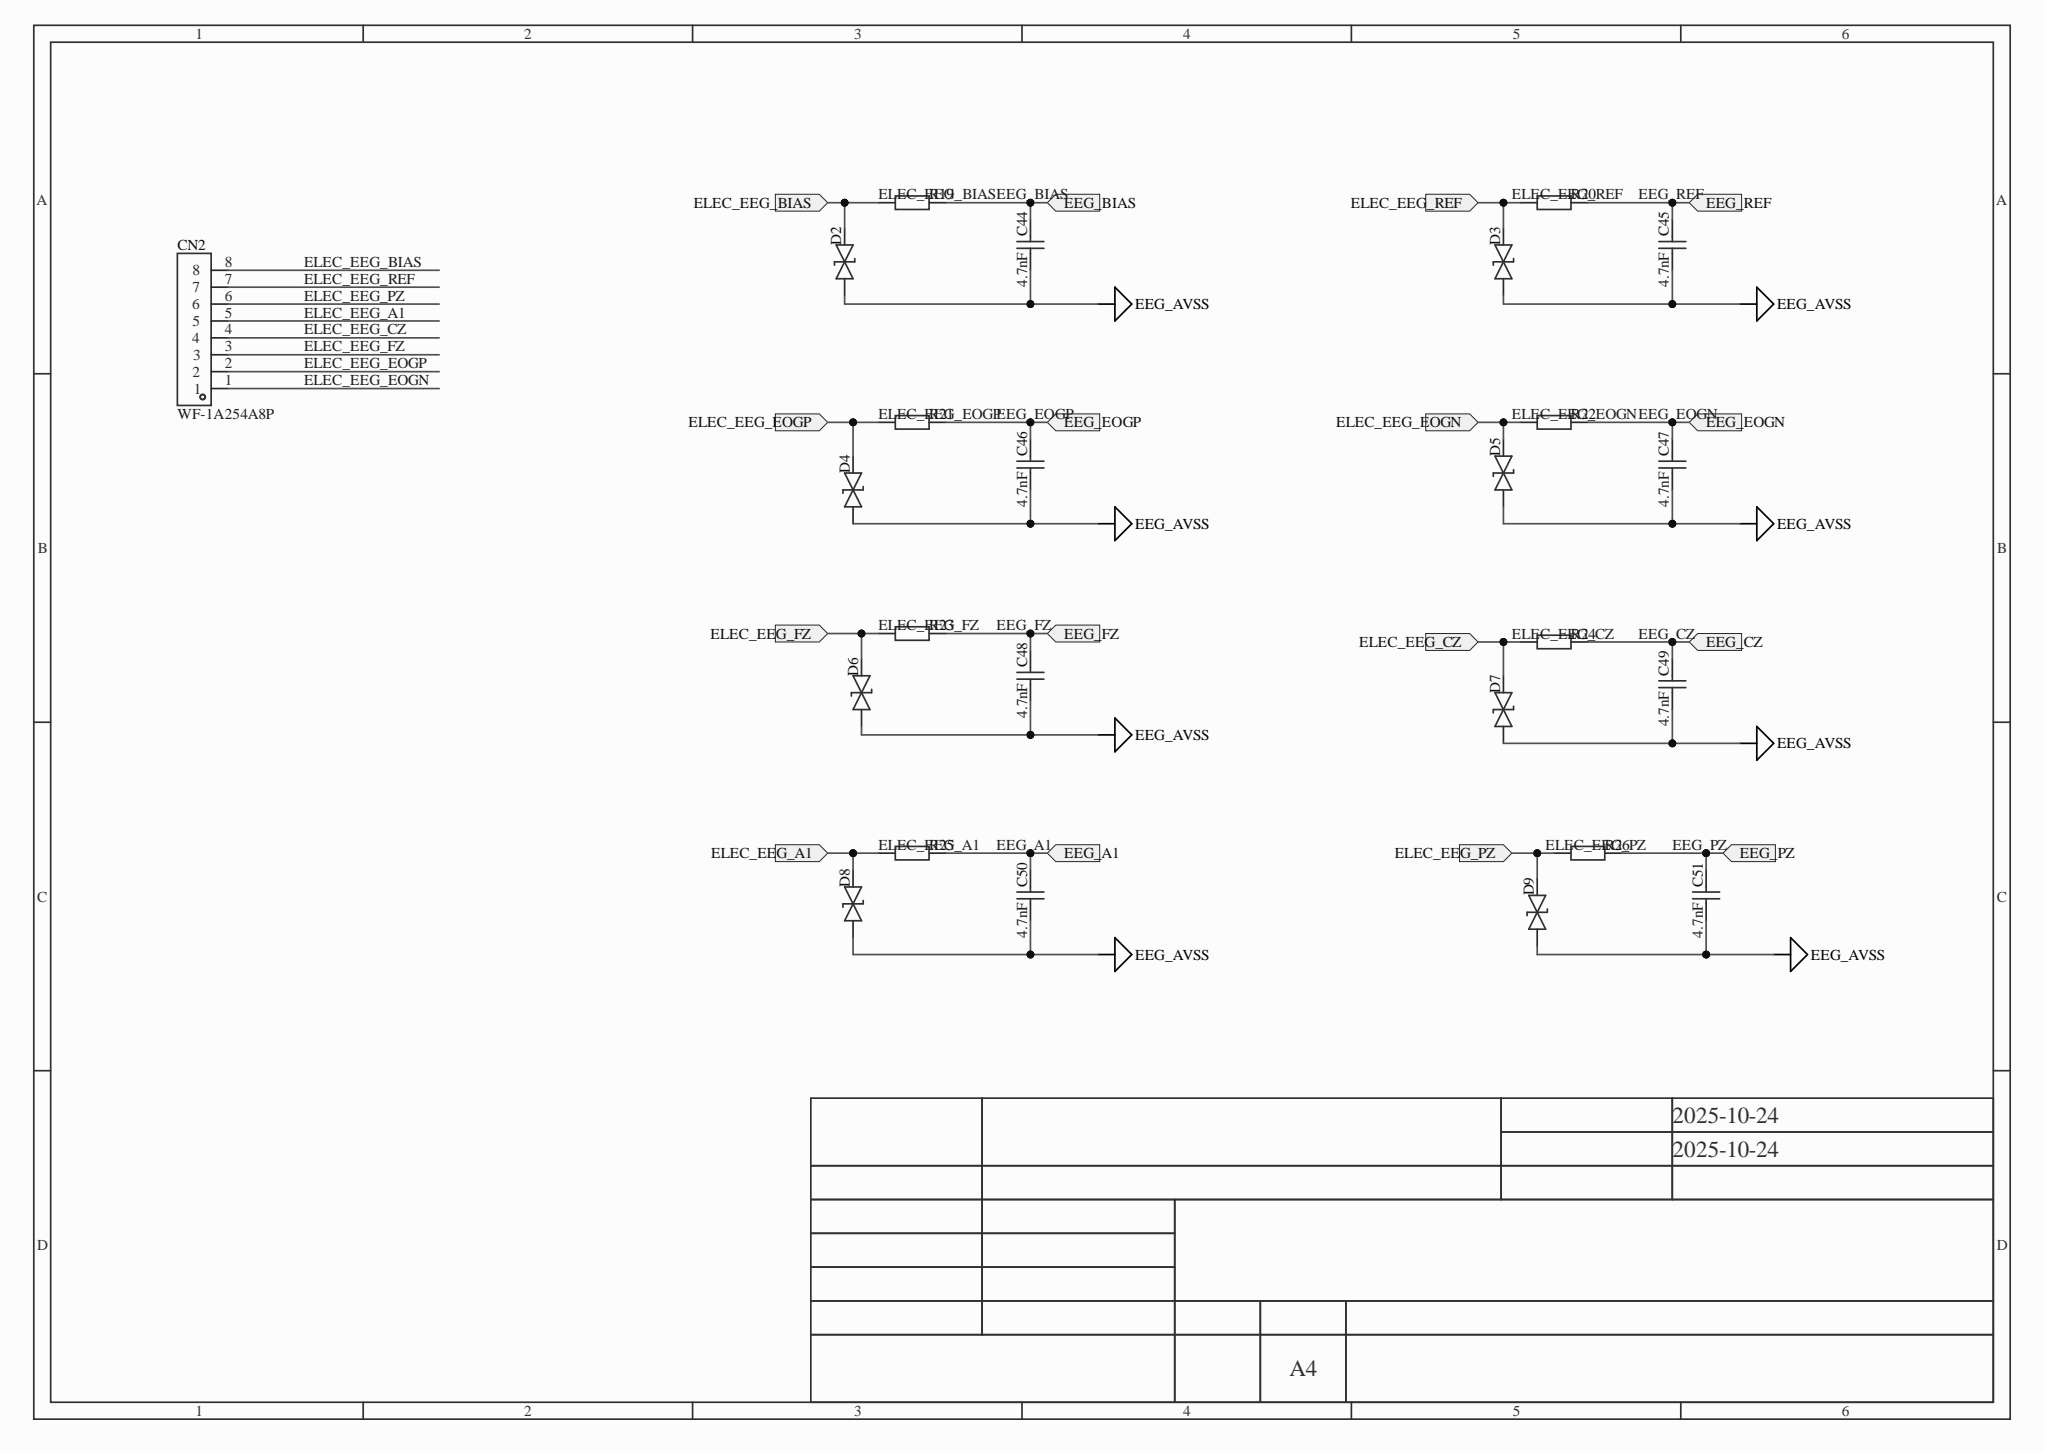Circuit board | Altium Designer | 212 parts | 123 nets | one sheet of the schematic
Parts on this sheet (reference | value | footprint):
C44 | 4.7nF | C0402
C45 | 4.7nF | C0402
C46 | 4.7nF | C0402
C47 | 4.7nF | C0402
C48 | 4.7nF | C0402
C49 | 4.7nF | C0402
C50 | 4.7nF | C0402
C51 | 4.7nF | C0402
CN2 | WF-1A254A8P | CONN-TH_WF-1A254A8P
D2 | TPD1E10B06DPYR-TP | X1-DFN1006-2_L1.0-W0.6-BI
D3 | TPD1E10B06DPYR-TP | X1-DFN1006-2_L1.0-W0.6-BI
D4 | TPD1E10B06DPYR-TP | X1-DFN1006-2_L1.0-W0.6-BI
D5 | TPD1E10B06DPYR-TP | X1-DFN1006-2_L1.0-W0.6-BI
D6 | TPD1E10B06DPYR-TP | X1-DFN1006-2_L1.0-W0.6-BI
D7 | TPD1E10B06DPYR-TP | X1-DFN1006-2_L1.0-W0.6-BI
D8 | TPD1E10B06DPYR-TP | X1-DFN1006-2_L1.0-W0.6-BI
D9 | TPD1E10B06DPYR-TP | X1-DFN1006-2_L1.0-W0.6-BI
R19 | R0402
R20 | R0402
R21 | R0402
R22 | R0402
R23 | R0402
R24 | R0402
R25 | R0402
R26 | R0402
Nets of these parts (net: part-pin ...):
ELEC_EEG_REF: CN2-7 D3-2 R20-1
ELEC_EEG_PZ: CN2-6 D9-2 R26-1
ELEC_EEG_FZ: CN2-3 D6-2 R23-1
ELEC_EEG_EOGP: CN2-2 D4-2 R21-1
ELEC_EEG_EOGN: CN2-1 D5-2 R22-1
ELEC_EEG_CZ: CN2-4 D7-2 R24-1
ELEC_EEG_BIAS: CN2-8 D2-2 R19-1
ELEC_EEG_A1: CN2-5 D8-2 R25-1
EEG_REF: C45-2 R20-2
EEG_PZ: C51-2 R26-2
EEG_FZ: C48-2 R23-2
EEG_EOGP: C46-2 R21-2
EEG_EOGN: C47-2 R22-2
EEG_CZ: C49-2 R24-2
EEG_BIAS: C44-2 R19-2
EEG_AVSS1: C44-1 C45-1 C46-1 C47-1 C48-1 C49-1 C50-1 C51-1 D2-1 D3-1 D4-1 D5-1 D6-1 D7-1 D8-1 D9-1
EEG_A1: C50-2 R25-2